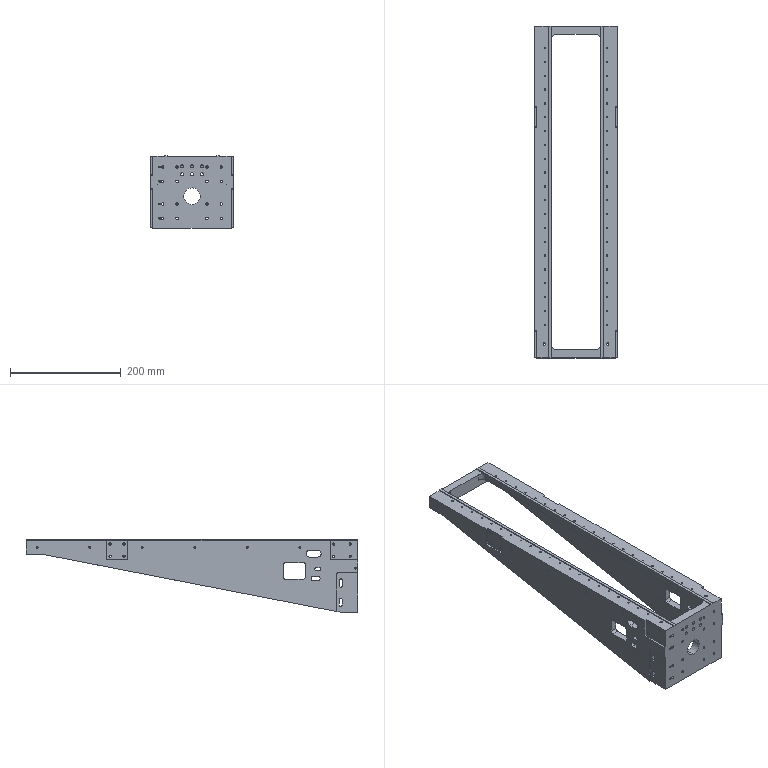Part | NX | features BREP 1 | 1 solid | 421 faces | box 150 x 600 x 131.5 mm | volume 1554104 mm3 | cylinder 278 | plane 72 | cone 71 | commonest cylinder face diameters 2.5 x108 4.2 x36 3.3 x32 4.5 x32 5.5 x24 8 x12